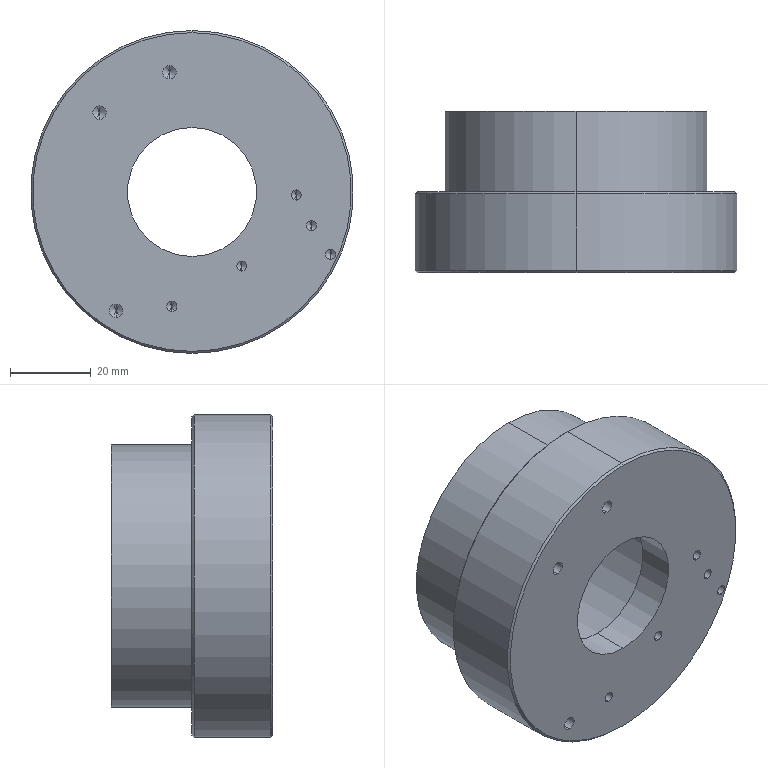Part | SolidWorks | features HoleWzd 5, Chamfer 1, RevCut 1, Revolution 1 | 1 solid | 75 faces | box 80 x 40 x 80 mm | volume 86830 mm3 | cylinder 38 | cone 32 | plane 5 | commonest cylinder face diameters 2.5 x22 3.3 x6 32 x2 45 x2 55 x2 65 x2